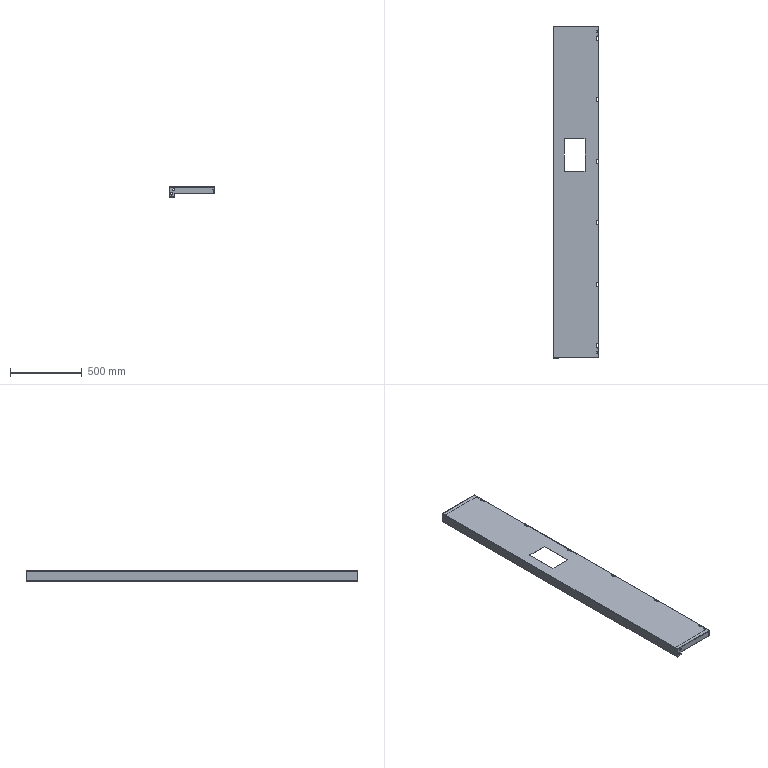Part | 3 solids | 234 faces | box 320 x 2316 x 70 mm | volume 1388899 mm3 | plane 146 | cylinder 88 | commonest cylinder face diameters 6.2 x28 9 x18 11 x10 3.4 x9 4 x8 8 x6